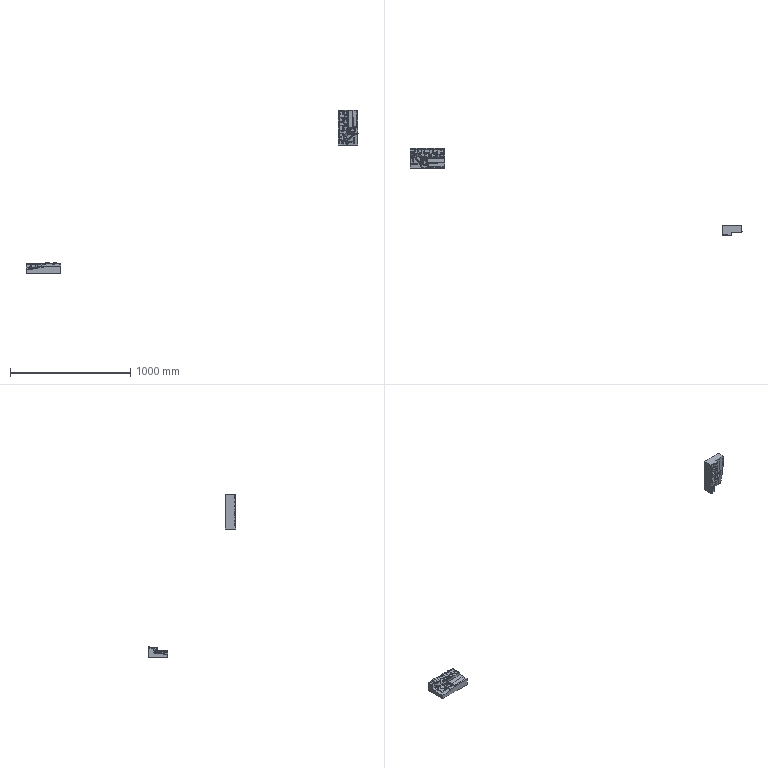NC program | NX | posted with a generic post | part box 2756 x 729.572 x 1353 mm
Lines 1 to 954 of 54396:
N10 G17 G21 G94 G90
(CAVITY_MILL_1 , TOOL : D30R5)
N12 T00 M6
N14 G54
N16 G17 G0 G90 X-143.25 Y-184.54 B0. C0. S3000 M3
N18 G43 Z97. H0
N20 Z88.645
N22 G94 G1 Z88.445 F2500.
N24 Y-164.04
N26 X-286.04
N28 Y-0.46
N30 X-0.46
N32 Y-164.04
N34 X-143.25
N36 Y-151.04
N38 X-273.04
N40 Y-13.46
N42 X-13.46
N44 Y-151.04
N46 X-143.25
N48 Y-138.04
N50 X-260.04
N52 Y-26.46
N54 X-26.46
N56 Y-138.04
N58 X-143.25
N60 Y-125.04
N62 X-247.04
N64 Y-39.46
N66 X-39.46
N68 Y-125.04
N70 X-143.25
N72 Y-112.04
N74 X-234.04
N76 Y-52.46
N78 X-52.46
N80 Y-112.04
N82 X-143.25
N84 Y-99.04
N86 X-221.04
N88 Y-65.46
N90 X-65.46
N92 Y-99.04
N94 X-143.25
N96 Y-86.04
N98 X-208.04
N100 Y-78.46
N102 X-78.46
N104 Y-86.04
N106 X-143.25
N108 Y-101.04
N110 Z88.645
N112 G0 Z89.3
N114 X-158.342 Y-185.392
N116 Z88.089
N118 G1 Z87.889
N120 Y-164.892
N122 X-286.731
N124 G2 X-286.892 Y-164.733 R0.159
N126 G1 Y0.228
N128 G2 X-286.729 Y0.392 R0.163
N130 G1 X-126.929
N132 G2 X-115.677 Y12.72 R17.729
N134 X-115.242 Y12.833 R2.6
N136 X-111.534 Y13.392 R103.881
N138 G1 X-91.854
N140 G2 X-82.268 Y0.768 R14.763
N142 X-82.264 Y0.392 R2.6
N144 G1 X-72.597
N146 X-72.598 Y0.545
N148 G2 X-72.582 Y0.835 R2.6
N150 G1 X-72.516 Y1.445
N152 G2 X-62.26 Y13.392 R13.928
N154 G1 X-47.094
N156 G2 X-37.691 Y11.42 R64.533
N158 X-36.883 Y11.024 R2.6
N160 X-29.841 Y0.392 R18.279
N162 G1 X0.231
N164 G2 X0.392 Y0.229 R0.163
N166 G1 Y-164.728
N168 G2 X0.236 Y-164.892 R0.156
N170 G1 X-158.342
N172 Y-151.892
N174 X-273.892
N176 Y-12.608
N178 X-126.929
N180 G3 X-125.299 Y-12.505 R13.
N182 X-116.107 Y-20.539 R17.729
N184 X-115.612 Y-20.675 R2.6
N186 X-96.003 Y-22.175 R106.601
N188 G1 X-95.841 Y-22.168
N190 G3 X-83.129 Y-12.579 R14.796
N192 G1 X-85.566 Y-11.672
N194 G2 X-96.044 Y-19.576 R12.196
N196 X-115.175 Y-18.111 R104.001
N198 X-114.808 Y10.269 R15.129
N200 X-96.044 Y11.675 R101.281
N202 X-84.859 Y0.553 R12.163
N204 G1 X-84.904 Y-0.114
N206 Y-7.446
N208 X-84.876 Y-8.779
N210 G2 X-85.566 Y-11.672 R12.196
N212 G1 X-83.129 Y-12.579
N214 G3 X-82.264 Y-12.608 R13.
N216 G1 X-72.597
N218 G3 X-71.856 Y-12.587 R13.
N220 X-59.04 Y-21.755 R14.323
N222 X-39.157 Y-19.831 R74.248
N224 X-38.445 Y-19.547 R2.6
N226 X-31.589 Y-12.49 R18.279
N228 G1 X-33.872 Y-11.247
N230 G2 X-39.753 Y-17.301 R15.679
N232 X-58.94 Y-19.157 R71.648
N234 X-69.904 Y-10.112 R11.723
N236 G1 X-69.969 Y-8.779
N238 X-69.998 Y0.553
N240 X-69.931 Y1.163
N242 G2 X-59.356 Y11.242 R11.328
N244 X-38.413 Y8.922 R61.933
N246 X-33.872 Y-11.247 R15.679
N248 G1 X-31.589 Y-12.49
N250 G3 X-29.841 Y-12.608 R13.
N252 G1 X-12.608
N254 Y-151.892
N256 X-158.342
N258 Y-138.892
N260 X-260.892
N262 Y-25.608
N264 X-131.588
N266 G3 X-120.769 Y-32.674 R30.729
N268 X-117.795 Y-33.49 R15.6
N270 X-95.795 Y-35.174 R119.601
N272 X-94.827 Y-35.128 R15.6
N274 X-77.417 Y-27.147 R27.796
N276 X-59.541 Y-34.745 R27.323
N278 X-36.176 Y-32.485 R87.248
N280 X-31.903 Y-30.781 R15.6
N282 X-25.608 Y-25.95 R31.279
N284 G1 Y-138.892
N286 X-158.342
N288 Y-125.892
N290 X-247.892
N292 Y-38.608
N294 X-136.466
N296 G3 X-125.43 Y-44.81 R43.729
N298 X-119.979 Y-46.305 R28.6
N300 X-95.587 Y-48.172 R132.601
N302 X-93.813 Y-48.089 R28.6
N304 X-77.268 Y-43.126 R40.796
N306 X-60.041 Y-47.735 R40.323
N308 X-38.608 Y-46.257 R100.248
N310 G1 Y-125.892
N312 X-158.342
N314 Y-112.892
N316 X-234.892
N318 Y-51.608
N320 X-140.582
N322 G3 X-130.092 Y-56.945 R56.729
N324 X-122.162 Y-59.12 R41.6
N326 X-95.379 Y-61.17 R145.601
N328 X-92.799 Y-61.049 R41.6
N330 X-77.117 Y-57.406 R53.796
N332 X-60.541 Y-60.726 R53.323
N334 X-51.608 Y-60.717 R113.248
N336 G1 Y-112.892
N338 X-158.342
N340 Y-99.892
N342 X-221.892
N344 Y-64.608
N346 X-144.209
N348 G3 X-134.753 Y-69.081 R69.729
N350 X-124.346 Y-71.936 R54.6
N352 X-95.172 Y-74.169 R158.601
N354 X-91.785 Y-74.009 R54.6
N356 X-76.967 Y-71.139 R66.796
N358 X-64.608 Y-73.482 R66.323
N360 G1 Y-99.892
N362 X-89.85
N364 Y-86.892
N366 G3 X-77.608 Y-84.822 R79.796
N368 G1 Y-86.892
N370 X-89.85
N372 Y-99.892
N374 X-158.342
N376 Y-86.892
N378 X-208.892
N380 Y-77.608
N382 X-147.49
N384 G3 X-139.415 Y-81.216 R82.729
N386 X-126.53 Y-84.751 R67.6
N388 X-107.792 Y-86.892 R171.601
N390 G1 X-158.342
N392 Y-101.892
N394 Z88.089
N396 G0 Z88.745
N398 X-165.938 Y-185.976
N400 Z87.534
N402 G1 Z87.334
N404 Y-165.476
N406 X-286.748
N408 G2 X-287.476 Y-164.73 R0.746
N410 G1 Y0.245
N412 G2 X-286.747 Y0.976 R0.73
N414 G1 X-138.064
N416 G2 X-126.86 Y13.976 R14.714
N418 G1 X-90.114
N420 G2 X-85.07 Y10.708 R18.091
N422 X-80.471 Y0.976 R14.239
N424 G1 X-74.622
N426 G2 X-66.421 Y13.261 R15.165
N428 X-64.844 Y13.976 R18.211
N430 G1 X-28.12
N432 G2 X-17.148 Y0.976 R14.841
N434 G1 X0.248
N436 G2 X0.976 Y0.247 R0.73
N438 G1 Y-164.745
N440 G2 X0.227 Y-165.476 R0.748
N442 G1 X-165.938
N444 Y-152.476
N446 X-274.476
N448 Y-12.024
N450 X-138.064
N452 G3 X-137.487 Y-12.011 R13.
N454 X-124.369 Y-22.242 R14.88
N456 X-98.056 Y-23.371 R606.524
N458 X-88.113 Y-20.877 R19.434
N460 X-81.054 Y-12.011 R15.061
N462 G1 X-83.548 Y-11.275
N464 G2 X-89.388 Y-18.612 R12.461
N466 X-98.001 Y-20.772 R16.834
N468 X-124.189 Y-19.648 R603.924
N470 X-135.543 Y-8.779 R12.28
N472 G1 X-135.505 Y-7.446
N474 X-135.49 Y0.553
N476 G2 X-124.189 Y11.762 R12.114
N478 X-97.384 Y12.861 R559.41
N480 X-86.826 Y8.791 R15.491
N482 X-83.051 Y0.227 R11.639
N484 G1 X-83.039 Y-7.734
N486 G2 X-83.548 Y-11.275 R12.461
N488 G1 X-81.054 Y-12.011
N490 G3 X-80.471 Y-12.024 R13.
N492 G1 X-74.622
N494 G3 X-74.06 Y-12.011 R13.
N496 X-71.249 Y-17.286 R15.219
N498 X-58.488 Y-23.139 R16.889
N500 X-31.615 Y-22.41 R839.093
N502 X-17.794 Y-12.008 R15.021
N504 G1 X-20.269 Y-11.209
N506 G2 X-31.712 Y-19.812 R12.421
N508 X-58.517 Y-20.539 R836.493
N510 X-69.239 Y-15.636 R14.289
N512 X-72.052 Y-8.779 R12.619
N514 G1 X-72.08 Y-7.446
N516 X-72.077 Y-0.78
N518 X-72.07 Y-0.114
N520 G2 X-65.235 Y10.947 R12.565
N522 X-57.866 Y12.662 R15.611
N524 X-33.052 Y11.993 R1140.581
N526 G1 X-31.005 Y11.838
N528 G2 X-19.722 Y0.553 R12.241
N530 G1 X-19.746 Y-8.779
N532 G2 X-20.269 Y-11.209 R12.421
N534 G1 X-17.794 Y-12.008
N536 G3 X-17.148 Y-12.024 R13.
N538 G1 X-12.024
N540 Y-152.476
N542 X-165.938
N544 Y-139.476
N546 X-261.476
N548 Y-25.024
N550 X-144.942
N552 G3 X-125.238 Y-35.213 R27.88
N554 X-98.332 Y-36.368 R619.524
N556 X-81.737 Y-32.206 R32.434
N558 X-77.508 Y-29.286 R28.061
N560 X-58.425 Y-36.139 R29.889
N562 X-31.119 Y-35.401 R852.093
N564 X-25.024 Y-34.512 R28.021
N566 G1 Y-139.476
N568 X-165.938
N570 Y-126.476
N572 X-248.476
N574 Y-38.024
N576 X-150.418
N578 G3 X-126.1 Y-48.184 R40.88
N580 X-98.607 Y-49.365 R632.524
N582 X-77.518 Y-44.674 R45.434
N584 X-58.345 Y-49.139 R42.889
N586 X-38.024 Y-48.678 R865.093
N588 G1 Y-126.476
N590 X-165.938
N592 Y-113.476
N594 X-235.476
N596 Y-51.024
N598 X-154.96
N600 G3 X-126.959 Y-61.156 R53.88
N602 X-98.883 Y-62.362 R645.524
N604 X-77.506 Y-58.795 R58.434
N606 X-58.256 Y-62.139 R55.889
N608 X-51.024 Y-62.03 R878.093
N610 G1 Y-113.476
N612 X-165.938
N614 Y-100.476
N616 X-222.476
N618 Y-64.024
N620 X-158.927
N622 G3 X-127.816 Y-74.127 R66.88
N624 X-99.158 Y-75.359 R658.524
N626 X-77.467 Y-72.466 R71.434
N628 X-64.024 Y-74.914 R68.889
N630 G1 Y-100.476
N632 X-85.357
N634 Y-87.476
N636 G3 X-77.415 Y-85.916 R84.434
N638 G1 X-77.024 Y-86.008
N640 Y-87.476
N642 X-85.357
N644 Y-100.476
N646 X-165.938
N648 Y-87.476
N650 X-209.476
N652 Y-77.024
N654 X-162.494
N656 G3 X-128.671 Y-87.099 R79.88
N658 X-122.4 Y-87.476 R671.524
N660 G1 X-104.006 Y-87.856
N662 X-122.4 Y-87.476
N664 X-165.938
N666 Y-102.476
N668 Z87.534
N670 G0 Z88.189
N672 X-170.954 Y-186.407
N674 Z86.978
N676 G1 Z86.778
N678 Y-165.907
N680 X-286.724
N682 G2 X-287.907 Y-164.725 R1.182
N684 G1 Y0.225
N686 G2 X-286.725 Y1.407 R1.182
N688 G1 X-254.472
N690 G2 X-241. Y13.843 R14.127
N692 G1 X-238.213 Y13.952
N694 G2 X-237.937 Y13.948 R2.6
N696 G1 X-224.038 Y13.016
N698 G2 X-212.026 Y1.407 R12.943
N700 G1 X-139.86
N702 G2 X-132.46 Y12.885 R15.157
N704 X-129.189 Y14.407 R18.937
N706 G1 X-89.044
N708 G2 X-86.625 Y13.141 R20.53
N710 X-79.246 Y1.407 R15.581
N712 G1 X-75.829
N714 G2 X-67.975 Y13.454 R15.751
N716 X-66.071 Y14.407 R19.393
N718 G1 X-25.97
N720 G2 X-19.793 Y10.349 R17.271
N722 X-15.619 Y1.407 R14.911
N724 G1 X0.224
N726 G2 X1.407 Y0.225 R1.182
N728 G1 Y-164.725
N730 G2 X0.225 Y-165.907 R1.182
N732 G1 X-170.954
N734 Y-152.907
N736 X-274.907
N738 Y-11.593
N740 X-254.472
N742 G3 X-254.009 Y-11.585 R13.
N744 X-241.341 Y-21.769 R14.275
N746 G1 X-239.637 Y-21.891
N748 G3 X-239.285 Y-21.892 R2.6
N750 G1 X-223.956 Y-20.91
N752 G3 X-213.775 Y-14.65 R12.762
N754 G1 X-213.086 Y-13.481
N756 G3 X-212.732 Y-12.328 R2.6
N758 G1 X-212.684 Y-11.576
N760 X-215.278 Y-11.41
N762 X-215.327 Y-12.161
N764 X-216.015 Y-13.331
N766 G2 X-224.122 Y-18.316 R10.162
N768 G1 X-239.451 Y-19.297
N770 X-241.156 Y-19.175
N772 G2 X-251.906 Y-8.979 R11.675
N774 G1 X-251.931 Y-8.779
N776 X-251.949 Y0.553
N778 X-251.908 Y0.943
N780 G2 X-240.898 Y11.245 R11.527
N782 G1 X-238.111 Y11.354
N784 X-224.212 Y10.422
N786 G2 X-214.581 Y-0.561 R10.343
N788 G1 X-215.278 Y-11.41
N790 X-212.684 Y-11.576
N792 G3 X-212.026 Y-11.593 R13.
N794 G1 X-139.86
N796 G3 X-139.486 Y-11.588 R13.
N798 X-134.972 Y-18.922 R14.435
N800 X-123.823 Y-23.375 R18.195
N802 G1 X-122.919 Y-23.42
N804 X-98.747 Y-24.065
N806 X-97.407 Y-24.076
N808 G3 X-86.904 Y-21.211 R21.051
N810 X-79.654 Y-11.587 R15.57
N812 G1 X-82.174 Y-10.948
N814 G2 X-88.214 Y-18.965 R12.97
N816 X-97.384 Y-21.476 R18.451
N818 G1 X-98.725 Y-21.465
N820 X-122.849 Y-20.82
N822 X-123.701 Y-20.778
N824 G2 X-133.265 Y-16.961 R15.595
N826 X-137.331 Y-8.053 R11.835
N828 G1 X-137.343 Y-0.206
N830 G2 X-131.143 Y10.643 R12.557
N832 X-123.515 Y12.879 R16.337
N834 X-97.384 Y13.553 R963.645
N836 X-87.98 Y10.923 R17.93
N838 X-81.767 Y-0.152 R12.981
N840 G1 X-81.766 Y-7.446
N842 X-81.78 Y-8.054
N844 G2 X-82.174 Y-10.948 R12.97
N846 G1 X-79.654 Y-11.587
N848 G3 X-79.246 Y-11.593 R13.
N850 G1 X-75.829
N852 G3 X-75.433 Y-11.587 R13.
N854 X-69.215 Y-20.53 R15.465
N856 X-58.509 Y-23.908 R19.132
N858 G1 X-57.13 Y-23.903
N860 X-32.125 Y-23.454
N862 G3 X-22.52 Y-20.542 R18.39
N864 X-16.04 Y-11.586 R15.141
N866 G1 X-18.557 Y-10.936
N868 G2 X-23.924 Y-18.354 R12.541
N870 X-32.171 Y-20.854 R15.79
N872 G1 X-57.177 Y-21.303
N874 X-58.517 Y-21.308
N876 G2 X-67.74 Y-18.389 R16.532
N878 X-73.302 Y-8.083 R12.865
N880 G1 X-73.316 Y-7.446
N882 X-73.313 Y-0.219
N884 G2 X-66.685 Y11.196 R13.151
N886 X-58.517 Y13.407 R16.793
N888 X-31.712 Y12.942 R1207.298
N890 X-21.652 Y8.532 R14.671
N892 X-18.146 Y-0.074 R12.311
N894 G1 Y-7.446
N896 X-18.162 Y-8.107
N898 G2 X-18.557 Y-10.936 R12.541
N900 G1 X-16.04 Y-11.586
N902 G3 X-15.619 Y-11.593 R13.
N904 G1 X-11.593
N906 Y-152.907
N908 X-170.954
N910 Y-139.907
N912 X-261.907
N914 Y-24.593
N916 X-261.6
N918 G3 X-242.27 Y-34.735 R27.275
N920 G1 X-240.566 Y-34.857
N922 G3 X-238.454 Y-34.865 R15.6
N924 G1 X-223.125 Y-33.884
N926 G3 X-204.92 Y-24.593 R25.762
N928 G1 X-147.37
N930 G3 X-143.507 Y-28.729 R27.435
N932 X-124.438 Y-36.36 R31.195
N934 G1 X-123.554 Y-36.405
N936 X-123.342 Y-36.413
N938 X-99.083 Y-37.061
N940 X-98.919 Y-37.064
N942 X-97.433 Y-37.077
N944 G3 X-80.357 Y-32.442 R34.051
N946 X-77.529 Y-30.56 R28.57
N948 X-76.592 Y-31.234 R28.465
N950 X-58.54 Y-36.908 R32.132
N952 G1 X-57.081 Y-36.903
N954 X-56.945 Y-36.902
N956 X-31.891 Y-36.451
N958 G3 X-24.593 Y-35.456 R31.39
N960 G1 Y-139.907
N962 X-170.954
N964 Y-126.907
N966 X-248.907
N968 Y-46.879
N970 G3 X-243.199 Y-47.702 R40.275
N972 G1 X-241.494 Y-47.824
N974 G3 X-237.624 Y-47.839 R28.6
N976 G1 X-222.295 Y-46.857
N978 G3 X-199.532 Y-37.593 R38.762
N980 G1 X-153.086
N982 G3 X-152.041 Y-38.535 R40.435
N984 X-125.06 Y-49.346 R44.195
N986 G1 X-124.129 Y-49.392
N988 X-123.765 Y-49.406
N990 X-99.371 Y-50.058
N992 X-99.09 Y-50.063
N994 X-97.475 Y-50.077
N996 G3 X-77.54 Y-45.629 R47.051
N998 X-58.557 Y-49.908 R45.132
N1000 G1 X-56.993 Y-49.903
N1002 X-56.76 Y-49.901
N1004 X-37.593 Y-49.556
N1006 Y-126.907
N1008 X-170.954
N1010 Y-113.907
N1012 X-235.907
N1014 Y-60.756
N1016 X-221.464 Y-59.831
N1018 G3 X-195.107 Y-50.593 R51.762
N1020 G1 X-157.82
N1022 G3 X-125.686 Y-62.331 R57.195
N1024 G1 X-124.704 Y-62.38
N1026 X-124.188 Y-62.4
N1028 X-99.66 Y-63.055
N1030 X-99.262 Y-63.062
N1032 X-97.527 Y-63.077
N1034 G3 X-77.53 Y-59.656 R60.051
N1036 X-58.566 Y-62.908 R58.132
N1038 G1 X-56.904 Y-62.903
N1040 X-56.575 Y-62.899
N1042 X-50.593 Y-62.792
N1044 Y-113.907
N1046 X-170.954
N1048 Y-100.907
N1050 X-222.907
N1052 Y-72.95
N1054 X-220.633 Y-72.804
N1056 G3 X-191.262 Y-63.593 R64.762
N1058 G1 X-161.98
N1060 G3 X-126.315 Y-75.315 R70.195
N1062 G1 X-125.279 Y-75.367
N1064 X-124.611 Y-75.393
N1066 X-99.948 Y-76.052
N1068 X-99.433 Y-76.061
N1070 X-97.586 Y-76.077
N1072 G3 X-77.502 Y-73.284 R73.051
N1074 X-63.593 Y-75.715 R71.132
N1076 G1 Y-100.907
N1078 X-83.367
N1080 Y-87.907
N1082 G3 X-77.465 Y-86.71 R86.051
N1084 X-76.593 Y-86.908 R84.132
N1086 G1 Y-87.907
N1088 X-83.367
N1090 Y-100.907
N1092 X-170.954
N1094 Y-87.907
N1096 X-209.907
N1098 Y-84.503
N1100 G3 X-187.815 Y-76.593 R77.762
N1102 G1 X-165.736
N1104 G3 X-132. Y-87.907 R83.195
N1106 G1 X-122.461 Y-90.907
N1108 X-92.907
N1110 G2 X-93.177 Y-85.964 R10.
N1112 X-97.673 Y-86.076 R83.051
N1114 G1 X-99.52 Y-86.06
N1116 X-99.61 Y-86.059
N1118 X-100.125 Y-86.05
N1120 X-100.215 Y-86.048
N1122 X-122.305 Y-85.458
N1124 G2 X-122.461 Y-90.907 R10.
N1126 G1 X-132. Y-87.907
N1128 X-170.954
N1130 Y-102.907
N1132 Z86.978
N1134 G0 Z87.634
N1136 X-172.587 Y-186.729
N1138 Z86.423
N1140 G1 Z86.223
N1142 Y-166.229
N1144 X-286.706
N1146 G2 X-288.014 Y-165.481 R1.543
N1148 X-288.173 Y-165.096 R1.361
N1150 G1 X-288.229 Y-164.287
N1152 Y0.211
N1154 G2 X-287.314 Y1.596 R1.524
N1156 X-286.666 Y1.729 R1.835
N1158 G1 X-257.125
N1160 G2 X-249.181 Y12.955 R14.838
N1162 X-244.324 Y14.729 R21.07
N1164 G1 X-222.246
N1166 X-221.675 Y14.649
N1168 G2 X-208.739 Y4.072 R15.949
N1170 X-208.626 Y3.62 R2.6
N1172 X-208.367 Y1.729 R51.005
N1174 G1 X-141.07
N1176 G2 X-135.033 Y12.247 R15.311
N1178 X-130.624 Y14.729 R19.538
N1180 G1 X-88.175
N1182 G2 X-86.703 Y14.011 R22.745
N1184 X-78.291 Y1.729 R16.106
N1186 G1 X-76.736
N1188 G2 X-69.103 Y13.591 R16.007
N1190 X-66.937 Y14.729 R20.725
N1192 G1 X-24.759
N1194 G2 X-20.904 Y12.564 R19.165
N1196 X-14.556 Y1.729 R15.63
N1198 G1 X0.211
N1200 G2 X1.596 Y0.815 R1.524
N1202 X1.729 Y0.158 R1.908
N1204 G1 Y-164.711
N1206 G2 X0.83 Y-166.09 R1.524
N1208 X0.14 Y-166.229 R2.054
N1210 G1 X-172.587
N1212 Y-153.229
N1214 X-275.229
N1216 Y-11.271
N1218 X-257.125
N1220 G3 X-256.863 Y-11.269 R13.
N1222 X-251.946 Y-18.98 R13.982
N1224 X-239.405 Y-23.165 R19.397
N1226 G1 X-238.056 Y-23.152
N1228 X-224.654 Y-22.871
N1230 G3 X-216.505 Y-20.902 R20.511
N1232 X-208.618 Y-11.269 R14.557
N1234 G1 X-211.141 Y-10.64
N1236 G2 X-217.619 Y-18.553 R11.957
N1238 X-224.709 Y-20.271 R17.911
N1240 G1 X-238.111 Y-20.553
N1242 X-239.451 Y-20.565
N1244 G2 X-250.331 Y-16.942 R16.797
N1246 X-254.646 Y-8.036 R11.382
N1248 G1 X-254.658 Y-0.271
N1250 G2 X-247.996 Y10.641 R12.238
N1252 X-239.451 Y12.669 R18.47
N1254 G1 X-224.709 Y12.371
N1256 X-223.368 Y12.26
N1258 X-222.028 Y12.073
N1260 G2 X-211.195 Y3.219 R13.349
N1262 X-210.842 Y-8.9 R48.405
N1264 X-211.141 Y-10.64 R11.957
N1266 G1 X-208.618 Y-11.269
N1268 G3 X-208.367 Y-11.271 R13.
N1270 G1 X-141.07
N1272 G3 X-140.774 Y-11.268 R13.
N1274 X-132.73 Y-21.643 R15.674
N1276 X-123.231 Y-24.094 R21.835
N1278 X-97.554 Y-24.574 R1750.844
N1280 X-87.416 Y-22.258 R22.244
N1282 X-78.587 Y-11.268 R16.074
N1284 G1 X-81.122 Y-10.693
N1286 G2 X-88.274 Y-19.782 R13.474
N1288 G1 X-88.572 Y-19.929
N1290 G2 X-97.524 Y-21.974 R19.644
N1292 X-123.164 Y-21.495 R1748.244
N1294 X-131.531 Y-19.335 R19.235
N1296 X-138.578 Y-7.719 R13.074
N1298 G1 X-138.569 Y0.003
N1300 G2 X-133.475 Y10.166 R12.711
N1302 X-124.189 Y13.521 R16.938
N1304 X-97.384 Y14.085 R1157.07
N1306 X-87.926 Y11.717 R20.145
N1308 X-80.775 Y-0.208 R13.506
N1310 G1 X-80.778 Y-7.446
N1312 X-80.792 Y-8.031
N1314 G2 X-81.122 Y-10.693 R13.474
N1316 G1 X-78.587 Y-11.268
N1318 G3 X-78.291 Y-11.271 R13.
N1320 G1 X-76.736
N1322 G3 X-76.453 Y-11.268 R13.
N1324 X-69.349 Y-21.318 R15.933
N1326 X-58.512 Y-24.462 R20.662
N1328 G1 X-57.143 Y-24.459
N1330 X-32.987 Y-24.149
N1332 X-31.647 Y-24.116
N1334 G3 X-22.192 Y-21.319 R20.01
N1336 X-14.858 Y-11.268 R15.83
N1338 G1 X-17.392 Y-10.684
N1340 G2 X-23.521 Y-19.085 R13.23
N1342 X-31.712 Y-21.517 R17.41
N1344 G1 X-33.052 Y-21.55
N1346 X-57.177 Y-21.859
N1348 X-58.517 Y-21.862
N1350 G2 X-67.97 Y-19.113 R18.062
N1352 X-74.229 Y-8.113 R13.333
N1354 G1 X-74.244 Y-7.446
N1356 X-74.242 Y-0.112
N1358 G2 X-67.76 Y11.364 R13.407
N1360 X-58.517 Y13.969 R18.125
N1362 X-31.712 Y13.607 R1815.86
N1364 X-22.431 Y10.459 R16.565
N1366 X-17.049 Y-0.079 R13.03
N1368 G1 X-17.043 Y-7.446
N1370 X-17.058 Y-8.045
N1372 G2 X-17.392 Y-10.684 R13.23
N1374 G1 X-14.858 Y-11.268
N1376 G3 X-14.556 Y-11.271 R13.
N1378 G1 X-11.271
N1380 Y-153.229
N1382 X-172.587
N1384 Y-140.229
N1386 X-262.229
N1388 Y-27.212
N1390 G3 X-260.017 Y-29.17 R26.982
N1392 X-239.193 Y-36.164 R32.397
N1394 G1 X-237.93 Y-36.152
N1396 X-237.822 Y-36.15
N1398 X-224.314 Y-35.866
N1400 G3 X-210.935 Y-32.648 R33.511
N1402 X-200.688 Y-24.271 R27.557
N1404 G1 X-148.928
N1406 G3 X-138.724 Y-33.178 R28.674
N1408 X-123.569 Y-37.09 R34.835
N1410 X-97.701 Y-37.573 R1763.844
N1412 X-81.755 Y-33.961 R35.244
N1414 X-77.526 Y-31.488 R29.074
N1416 X-76.243 Y-32.339 R28.933
N1418 X-58.538 Y-37.462 R33.662
N1420 G1 X-57.113 Y-37.459
N1422 X-57.013 Y-37.458
N1424 X-32.813 Y-37.148
N1426 X-32.702 Y-37.146
N1428 X-31.234 Y-37.11
N1430 G3 X-24.271 Y-36.109 R33.01
N1432 G1 Y-140.229
N1434 X-172.587
N1436 Y-127.229
N1438 X-249.229
N1440 Y-48.203
N1442 G3 X-238.998 Y-49.162 R45.397
N1444 G1 X-237.772 Y-49.151
N1446 X-237.587 Y-49.148
N1448 X-223.987 Y-48.862
N1450 G3 X-205.364 Y-44.394 R46.511
N1452 X-194.935 Y-37.271 R40.557
N1454 G1 X-154.902
N1456 G3 X-144.718 Y-44.714 R41.674
N1458 X-123.907 Y-50.086 R47.835
N1460 X-97.849 Y-50.572 R1776.844
N1462 X-77.551 Y-46.347 R48.244
N1464 X-58.555 Y-50.462 R46.662
N1466 G1 X-57.053 Y-50.459
N1468 X-56.882 Y-50.458
N1470 X-37.271 Y-50.207
N1472 Y-127.229
N1474 X-172.587
N1476 Y-114.229
N1478 X-236.229
N1480 Y-62.123
N1482 X-223.599 Y-61.856
N1484 G3 X-199.794 Y-56.14 R59.511
N1486 X-190.182 Y-50.271 R53.557
N1488 G1 X-159.852
N1490 G3 X-150.711 Y-56.25 R54.674
N1492 X-124.245 Y-63.081 R60.835
N1494 X-97.996 Y-63.571 R1789.844
N1496 X-77.549 Y-60.303 R61.244
N1498 X-58.566 Y-63.462 R59.662
N1500 G1 X-56.994 Y-63.459
N1502 X-56.751 Y-63.457
N1504 X-50.271 Y-63.374
N1506 Y-114.229
N1508 X-172.587
N1510 Y-101.229
N1512 X-223.229
N1514 Y-74.851
N1516 G3 X-194.223 Y-67.886 R72.511
N1518 X-186.04 Y-63.271 R66.557
N1520 G1 X-164.174
N1522 G3 X-156.705 Y-67.786 R67.674
N1524 X-124.583 Y-76.077 R73.835
N1526 X-98.143 Y-76.571 R1802.844
N1528 X-77.534 Y-73.895 R74.244
N1530 X-63.271 Y-76.298 R72.662
N1532 G1 Y-101.229
N1534 X-82.032
N1536 Y-88.229
N1538 G3 X-77.511 Y-87.301 R87.244
N1540 X-76.271 Y-87.575 R85.662
N1542 G1 Y-88.229
N1544 X-82.032
N1546 Y-101.229
N1548 X-172.587
N1550 Y-88.229
N1552 X-210.229
N1554 Y-86.543
N1556 G3 X-188.652 Y-79.632 R85.511
N1558 X-182.32 Y-76.271 R79.557
N1560 G1 X-168.058
N1562 G3 X-162.699 Y-79.322 R80.674
N1564 X-134.946 Y-88.229 R86.835
N1566 G1 X-125.406 Y-91.229
N1568 X-91.571
N1570 G2 X-91.863 Y-86.4 R10.
N1572 X-98.257 Y-86.57 R84.244
N1574 X-124.844 Y-86.073 R1812.844
N1576 G1 X-125.183 Y-86.064
N1578 G2 X-125.406 Y-91.229 R10.
N1580 G1 X-134.946 Y-88.229
N1582 X-172.587
N1584 Y-103.229
N1586 Z86.423
N1588 G0 Z87.078
N1590 X-173.739 Y-186.964
N1592 Z85.868
N1594 G1 Z85.668
N1596 Y-166.464
N1598 X-286.722
N1600 G2 X-288.464 Y-164.722 R1.753
N1602 G1 Y0.222
N1604 G2 X-286.722 Y1.964 R1.753
N1606 G1 X-258.803
N1608 G2 X-251.441 Y12.923 R15.181
N1610 X-246.829 Y14.964 R22.391
N1612 G1 X-218.771
N1614 G2 X-213.84 Y12.878 R21.984
N1616 X-206.436 Y1.964 R15.082
N1618 G1 X-191.725
N1620 G2 X-182.923 Y12.343 R13.344
N1622 G1 X-182.793 Y12.384
N1624 X-181.743 Y12.686
N1626 G2 X-171.045 Y14.082 R36.012
N1628 G1 X-170.934 Y14.077
N1630 G2 X-157.588 Y1.964 R14.443
N1632 G1 X-142.038
N1634 G2 X-134.661 Y13.408 R16.04
N1636 X-131.679 Y14.964 R21.325
N1638 G1 X-87.365
N1640 X-87.261 Y14.917
N1642 G2 X-79.034 Y7.077 R17.366
N1644 X-77.467 Y2.017 R15.149
N1646 X-69.189 Y14.206 R16.417
N1648 X-67.698 Y14.964 R21.846
N1650 G1 X-23.803
N1652 G2 X-21.047 Y13.492 R20.743
N1654 X-13.716 Y1.964 R16.081
N1656 G1 X0.222
N1658 G2 X1.964 Y0.222 R1.753
N1660 G1 Y-164.722
N1662 G2 X0.221 Y-166.464 R1.753
N1664 G1 X-173.739
N1666 Y-153.464
N1668 X-275.464
N1670 Y-11.036
N1672 X-258.803
N1674 X-258.567 Y-11.034
N1676 G3 X-250.207 Y-21.523 R15.414
N1678 X-239.43 Y-23.93 R24.427
N1680 G1 X-238.073 Y-23.921
N1682 X-225.996 Y-23.743
N1684 X-224.669 Y-23.716
N1686 G3 X-214.064 Y-20.907 R22.306
N1688 X-206.658 Y-11.034 R15.137
N1690 G1 X-209.194 Y-10.458
N1692 G2 X-215.327 Y-18.635 R12.537
N1694 X-224.709 Y-21.116 R19.706
N1696 G1 X-226.049 Y-21.144
N1698 X-238.111 Y-21.321
N1700 X-239.451 Y-21.33
N1702 G2 X-249.081 Y-19.179 R21.827
N1704 X-256.348 Y-7.641 R12.814
N1706 G1 X-256.355 Y-0.192
N1708 G2 X-250.127 Y10.679 R12.581
N1710 X-240.792 Y13.378 R19.791
N1712 G1 X-239.451 Y13.417
N1714 X-224.709 Y13.241
N1716 X-223.368 Y13.155
N1718 G2 X-215.137 Y10.625 R19.384
N1720 X-208.881 Y-0.198 R12.482
N1722 G1 X-208.884 Y-7.446
N1724 G2 X-209.194 Y-10.458 R12.537
N1726 G1 X-206.658 Y-11.034
N1728 X-206.436 Y-11.036
N1730 X-191.725
N1732 X-191.526 Y-11.035
N1734 G3 X-181.064 Y-20.748 R13.037
N1736 G1 X-174.216 Y-21.916
N1738 G3 X-173.975 Y-21.945 R2.6
N1740 G1 X-172.762 Y-22.037
N1742 G3 X-157.847 Y-11.034 R14.525
N1744 G1 X-160.37 Y-10.408
N1746 G2 X-172.565 Y-19.445 R11.925
N1748 G1 X-173.779 Y-19.353
N1750 X-180.627 Y-18.185
N1752 G2 X-189.31 Y-7.897 R10.437
N1754 G1 Y0.
N1756 G2 X-182.074 Y9.885 R10.744
N1758 G1 X-181.025 Y10.187
N1760 G2 X-171.098 Y11.482 R33.412
N1762 X-160.037 Y0.553 R11.843
N1764 G1 X-160.076 Y-0.114
N1766 X-160.084 Y-8.779
N1768 G2 X-160.37 Y-10.408 R11.925
N1770 G1 X-157.847 Y-11.034
N1772 G3 X-157.588 Y-11.036 R13.
N1774 G1 X-142.038
N1776 X-141.823 Y-11.034
N1778 G3 X-134.082 Y-21.656 R16.063
N1780 X-123.474 Y-24.586 R22.242
N1782 G1 X-118.865 Y-24.676
N1784 X-98.189 Y-24.965
N1786 G3 X-92.089 Y-24.407 R29.175
N1788 X-83.854 Y-20.743 R20.44
N1790 X-77.679 Y-10.981 R16.146
N1792 G1 X-80.228 Y-10.469
N1794 G2 X-85.408 Y-18.659 R13.546
N1796 X-92.596 Y-21.857 R17.84
N1798 X-98.152 Y-22.365 R26.575
N1800 G1 X-118.828 Y-22.076
N1802 X-123.423 Y-21.986
N1804 G2 X-132.791 Y-19.399 R19.642
N1806 X-139.567 Y-8.011 R13.463
N1808 G1 X-139.58 Y-7.446
N1810 X-139.582 Y-0.188
N1812 G2 X-133.281 Y11.205 R13.44
N1814 X-123.78 Y14.058 R18.725
N1816 X-97.384 Y14.46 R1553.085
N1818 X-88.34 Y12.551 R21.741
N1820 X-81.345 Y5.886 R14.766
N1822 X-79.949 Y0.13 R12.549
N1824 G1 X-79.951 Y-7.446
N1826 X-79.967 Y-8.113
N1828 G2 X-80.228 Y-10.469 R13.546
N1830 G1 X-77.679 Y-10.981
N1832 G3 X-77.323 Y-10.982 R13.
N1834 X-76.487 Y-13.762 R15.156
N1836 X-67.621 Y-22.894 R17.04
N1838 X-58.505 Y-24.871 R22.266
N1840 X-31.672 Y-24.604 R2528.441
N1842 X-20.916 Y-21.278 R20.674
N1844 X-13.92 Y-11.035 R16.081
N1846 G1 X-16.466 Y-10.51
N1848 G2 X-22.331 Y-19.097 R13.481
N1850 X-31.712 Y-22.004 R18.074
N1852 X-58.517 Y-22.271 R2525.841
N1854 X-66.559 Y-20.521 R19.666
N1856 X-74.081 Y-12.779 R14.44
N1858 X-75.014 Y-8.02 R12.556
N1860 G1 X-75.008 Y-0.122
N1862 G2 X-67.922 Y11.935 R13.817
N1864 X-58.517 Y14.373 R19.246
N1866 X-31.712 Y14.118 R2677.998
N1868 X-22.44 Y11.297 R18.143
N1870 X-16.185 Y-0.074 R13.481
N1872 G1 X-16.18 Y-7.446
N1874 X-16.191 Y-8.042
N1876 G2 X-16.466 Y-10.51 R13.481
N1878 G1 X-13.92 Y-11.035
N1880 X-13.716 Y-11.036
N1882 X-11.036
N1884 Y-153.464
N1886 X-173.739
N1888 Y-140.464
N1890 X-262.464
N1892 Y-28.818
N1894 G3 X-255.835 Y-33.242 R28.414
N1896 X-239.334 Y-36.93 R37.427
N1898 G1 X-237.908 Y-36.92
N1900 X-225.75 Y-36.741
N1902 X-224.461 Y-36.715
N1904 G3 X-207.747 Y-32.27 R35.306
N1906 X-198.895 Y-24.541 R28.137